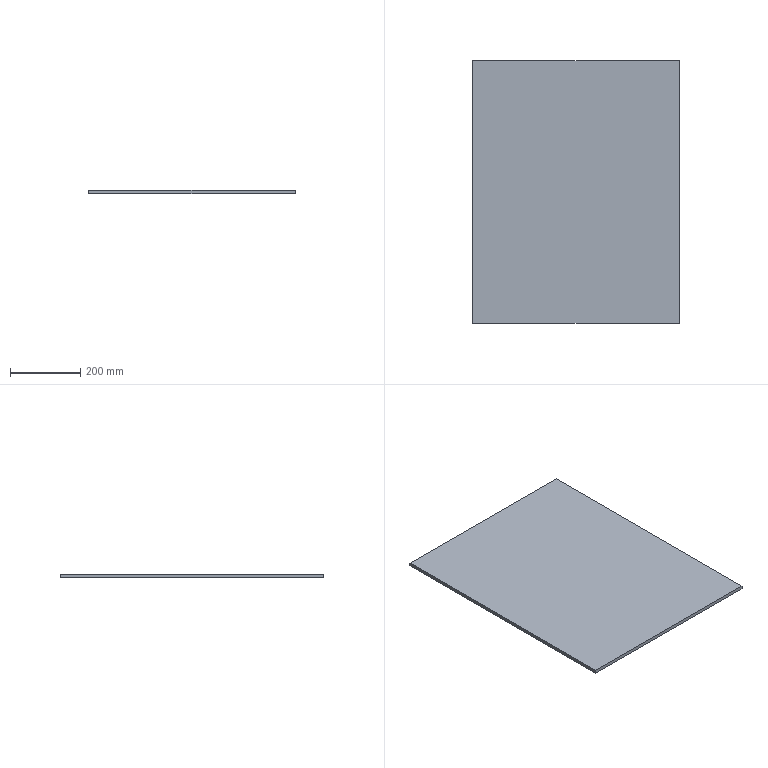Part | STEP file | floor | 1 solid | 6 faces | box 586.14 x 746.049 x 10 mm | volume 4372895 mm3 | plane 6
STEP:
#1=CARTESIAN_POINT('',(0.,0.,0.));
#2=DIRECTION('',(0.,0.,1.));
#3=DIRECTION('',(1.,0.,0.));
#4=AXIS2_PLACEMENT_3D('',#1,#2,#3);
#5=CARTESIAN_POINT('',(36.295,-184.35,-10.));
#6=VERTEX_POINT('',#5);
#7=CARTESIAN_POINT('',(36.295,561.699,-10.));
#8=VERTEX_POINT('',#7);
#9=CARTESIAN_POINT('',(36.295,-184.35,-10.));
#10=DIRECTION('',(0.,1.,0.));
#11=VECTOR('',#10,1.);
#12=LINE('',#9,#11);
#13=CARTESIAN_POINT('',(36.295,-184.35,0.));
#14=DIRECTION('',(1.,0.,0.));
#15=DIRECTION('',(0.,0.,-1.));
#16=AXIS2_PLACEMENT_3D('',#13,#14,#15);
#17=PLANE('',#16);
#18=CARTESIAN_POINT('',(10.,0.));
#19=DIRECTION('',(0.,1.));
#20=VECTOR('',#19,1.);
#21=LINE('',#18,#20);
#22=(GEOMETRIC_REPRESENTATION_CONTEXT(2)PARAMETRIC_REPRESENTATION_CONTEXT()REPRESENTATION_CONTEXT('',''));
#23=DEFINITIONAL_REPRESENTATION('',(#21),#22);
#24=PCURVE('',#17,#23);
#25=CARTESIAN_POINT('',(-256.775,188.674,-10.));
#26=DIRECTION('',(0.,0.,1.));
#27=DIRECTION('',(1.,0.,0.));
#28=AXIS2_PLACEMENT_3D('',#25,#26,#27);
#29=PLANE('',#28);
#30=CARTESIAN_POINT('',(293.07,-373.025));
#31=DIRECTION('',(0.,1.));
#32=VECTOR('',#31,1.);
#33=LINE('',#30,#32);
#34=(GEOMETRIC_REPRESENTATION_CONTEXT(2)PARAMETRIC_REPRESENTATION_CONTEXT()REPRESENTATION_CONTEXT('',''));
#35=DEFINITIONAL_REPRESENTATION('',(#33),#34);
#36=PCURVE('',#29,#35);
#37=SURFACE_CURVE('',#12,(#24,#36),.PCURVE_S1.);
#38=EDGE_CURVE('',#6,#8,#37,.T.);
#39=ORIENTED_EDGE('',*,*,#38,.T.);
#40=CARTESIAN_POINT('',(36.295,561.699,0.));
#41=VERTEX_POINT('',#40);
#42=CARTESIAN_POINT('',(36.295,561.699,0.));
#43=DIRECTION('',(0.,0.,-1.));
#44=VECTOR('',#43,1.);
#45=LINE('',#42,#44);
#46=CARTESIAN_POINT('',(0.,746.049));
#47=DIRECTION('',(1.,0.));
#48=VECTOR('',#47,1.);
#49=LINE('',#46,#48);
#50=(GEOMETRIC_REPRESENTATION_CONTEXT(2)PARAMETRIC_REPRESENTATION_CONTEXT()REPRESENTATION_CONTEXT('',''));
#51=DEFINITIONAL_REPRESENTATION('',(#49),#50);
#52=PCURVE('',#17,#51);
#53=CARTESIAN_POINT('',(36.295,561.699,0.));
#54=DIRECTION('',(0.,1.,0.));
#55=DIRECTION('',(0.,0.,1.));
#56=AXIS2_PLACEMENT_3D('',#53,#54,#55);
#57=PLANE('',#56);
#58=CARTESIAN_POINT('',(0.,0.));
#59=DIRECTION('',(-1.,0.));
#60=VECTOR('',#59,1.);
#61=LINE('',#58,#60);
#62=(GEOMETRIC_REPRESENTATION_CONTEXT(2)PARAMETRIC_REPRESENTATION_CONTEXT()REPRESENTATION_CONTEXT('',''));
#63=DEFINITIONAL_REPRESENTATION('',(#61),#62);
#64=PCURVE('',#57,#63);
#65=SURFACE_CURVE('',#45,(#52,#64),.PCURVE_S1.);
#66=EDGE_CURVE('',#41,#8,#65,.T.);
#67=ORIENTED_EDGE('',*,*,#66,.F.);
#68=CARTESIAN_POINT('',(36.295,-184.35,0.));
#69=VERTEX_POINT('',#68);
#70=CARTESIAN_POINT('',(36.295,561.699,0.));
#71=DIRECTION('',(0.,-1.,0.));
#72=VECTOR('',#71,1.);
#73=LINE('',#70,#72);
#74=CARTESIAN_POINT('',(0.,746.049));
#75=DIRECTION('',(0.,-1.));
#76=VECTOR('',#75,1.);
#77=LINE('',#74,#76);
#78=(GEOMETRIC_REPRESENTATION_CONTEXT(2)PARAMETRIC_REPRESENTATION_CONTEXT()REPRESENTATION_CONTEXT('',''));
#79=DEFINITIONAL_REPRESENTATION('',(#77),#78);
#80=PCURVE('',#17,#79);
#81=CARTESIAN_POINT('',(-256.775,188.674,0.));
#82=DIRECTION('',(0.,0.,1.));
#83=DIRECTION('',(1.,0.,0.));
#84=AXIS2_PLACEMENT_3D('',#81,#82,#83);
#85=PLANE('',#84);
#86=CARTESIAN_POINT('',(293.07,373.025));
#87=DIRECTION('',(0.,-1.));
#88=VECTOR('',#87,1.);
#89=LINE('',#86,#88);
#90=(GEOMETRIC_REPRESENTATION_CONTEXT(2)PARAMETRIC_REPRESENTATION_CONTEXT()REPRESENTATION_CONTEXT('',''));
#91=DEFINITIONAL_REPRESENTATION('',(#89),#90);
#92=PCURVE('',#85,#91);
#93=SURFACE_CURVE('',#73,(#80,#92),.PCURVE_S1.);
#94=EDGE_CURVE('',#41,#69,#93,.T.);
#95=ORIENTED_EDGE('',*,*,#94,.T.);
#96=CARTESIAN_POINT('',(36.295,-184.35,0.));
#97=DIRECTION('',(0.,0.,-1.));
#98=VECTOR('',#97,1.);
#99=LINE('',#96,#98);
#100=CARTESIAN_POINT('',(0.,0.));
#101=DIRECTION('',(1.,0.));
#102=VECTOR('',#101,1.);
#103=LINE('',#100,#102);
#104=(GEOMETRIC_REPRESENTATION_CONTEXT(2)PARAMETRIC_REPRESENTATION_CONTEXT()REPRESENTATION_CONTEXT('',''));
#105=DEFINITIONAL_REPRESENTATION('',(#103),#104);
#106=PCURVE('',#17,#105);
#107=CARTESIAN_POINT('',(-549.845,-184.35,0.));
#108=DIRECTION('',(0.,-1.,0.));
#109=DIRECTION('',(0.,0.,-1.));
#110=AXIS2_PLACEMENT_3D('',#107,#108,#109);
#111=PLANE('',#110);
#112=CARTESIAN_POINT('',(0.,586.14));
#113=DIRECTION('',(1.,0.));
#114=VECTOR('',#113,1.);
#115=LINE('',#112,#114);
#116=(GEOMETRIC_REPRESENTATION_CONTEXT(2)PARAMETRIC_REPRESENTATION_CONTEXT()REPRESENTATION_CONTEXT('',''));
#117=DEFINITIONAL_REPRESENTATION('',(#115),#116);
#118=PCURVE('',#111,#117);
#119=SURFACE_CURVE('',#99,(#106,#118),.PCURVE_S1.);
#120=EDGE_CURVE('',#69,#6,#119,.T.);
#121=ORIENTED_EDGE('',*,*,#120,.T.);
#122=EDGE_LOOP('',(#39,#67,#95,#121));
#123=FACE_BOUND('',#122,.T.);
#124=ADVANCED_FACE('',(#123),#17,.T.);
#125=CARTESIAN_POINT('',(-549.845,561.699,-10.));
#126=VERTEX_POINT('',#125);
#127=CARTESIAN_POINT('',(36.295,561.699,-10.));
#128=DIRECTION('',(-1.,0.,0.));
#129=VECTOR('',#128,1.);
#130=LINE('',#127,#129);
#131=CARTESIAN_POINT('',(-10.,0.));
#132=DIRECTION('',(0.,-1.));
#133=VECTOR('',#132,1.);
#134=LINE('',#131,#133);
#135=(GEOMETRIC_REPRESENTATION_CONTEXT(2)PARAMETRIC_REPRESENTATION_CONTEXT()REPRESENTATION_CONTEXT('',''));
#136=DEFINITIONAL_REPRESENTATION('',(#134),#135);
#137=PCURVE('',#57,#136);
#138=CARTESIAN_POINT('',(293.07,373.025));
#139=DIRECTION('',(-1.,0.));
#140=VECTOR('',#139,1.);
#141=LINE('',#138,#140);
#142=(GEOMETRIC_REPRESENTATION_CONTEXT(2)PARAMETRIC_REPRESENTATION_CONTEXT()REPRESENTATION_CONTEXT('',''));
#143=DEFINITIONAL_REPRESENTATION('',(#141),#142);
#144=PCURVE('',#29,#143);
#145=SURFACE_CURVE('',#130,(#137,#144),.PCURVE_S1.);
#146=EDGE_CURVE('',#8,#126,#145,.T.);
#147=ORIENTED_EDGE('',*,*,#146,.T.);
#148=CARTESIAN_POINT('',(-549.845,561.699,0.));
#149=VERTEX_POINT('',#148);
#150=CARTESIAN_POINT('',(-549.845,561.699,0.));
#151=DIRECTION('',(0.,0.,-1.));
#152=VECTOR('',#151,1.);
#153=LINE('',#150,#152);
#154=CARTESIAN_POINT('',(0.,-586.14));
#155=DIRECTION('',(-1.,0.));
#156=VECTOR('',#155,1.);
#157=LINE('',#154,#156);
#158=(GEOMETRIC_REPRESENTATION_CONTEXT(2)PARAMETRIC_REPRESENTATION_CONTEXT()REPRESENTATION_CONTEXT('',''));
#159=DEFINITIONAL_REPRESENTATION('',(#157),#158);
#160=PCURVE('',#57,#159);
#161=CARTESIAN_POINT('',(-549.845,561.699,0.));
#162=DIRECTION('',(-1.,0.,0.));
#163=DIRECTION('',(0.,0.,1.));
#164=AXIS2_PLACEMENT_3D('',#161,#162,#163);
#165=PLANE('',#164);
#166=CARTESIAN_POINT('',(0.,0.));
#167=DIRECTION('',(-1.,0.));
#168=VECTOR('',#167,1.);
#169=LINE('',#166,#168);
#170=(GEOMETRIC_REPRESENTATION_CONTEXT(2)PARAMETRIC_REPRESENTATION_CONTEXT()REPRESENTATION_CONTEXT('',''));
#171=DEFINITIONAL_REPRESENTATION('',(#169),#170);
#172=PCURVE('',#165,#171);
#173=SURFACE_CURVE('',#153,(#160,#172),.PCURVE_S1.);
#174=EDGE_CURVE('',#149,#126,#173,.T.);
#175=ORIENTED_EDGE('',*,*,#174,.F.);
#176=CARTESIAN_POINT('',(-549.845,561.699,0.));
#177=DIRECTION('',(1.,0.,0.));
#178=VECTOR('',#177,1.);
#179=LINE('',#176,#178);
#180=CARTESIAN_POINT('',(0.,-586.14));
#181=DIRECTION('',(0.,1.));
#182=VECTOR('',#181,1.);
#183=LINE('',#180,#182);
#184=(GEOMETRIC_REPRESENTATION_CONTEXT(2)PARAMETRIC_REPRESENTATION_CONTEXT()REPRESENTATION_CONTEXT('',''));
#185=DEFINITIONAL_REPRESENTATION('',(#183),#184);
#186=PCURVE('',#57,#185);
#187=CARTESIAN_POINT('',(-293.07,373.025));
#188=DIRECTION('',(1.,0.));
#189=VECTOR('',#188,1.);
#190=LINE('',#187,#189);
#191=(GEOMETRIC_REPRESENTATION_CONTEXT(2)PARAMETRIC_REPRESENTATION_CONTEXT()REPRESENTATION_CONTEXT('',''));
#192=DEFINITIONAL_REPRESENTATION('',(#190),#191);
#193=PCURVE('',#85,#192);
#194=SURFACE_CURVE('',#179,(#186,#193),.PCURVE_S1.);
#195=EDGE_CURVE('',#149,#41,#194,.T.);
#196=ORIENTED_EDGE('',*,*,#195,.T.);
#197=ORIENTED_EDGE('',*,*,#66,.T.);
#198=EDGE_LOOP('',(#147,#175,#196,#197));
#199=FACE_BOUND('',#198,.T.);
#200=ADVANCED_FACE('',(#199),#57,.T.);
#201=CARTESIAN_POINT('',(-549.845,-184.35,-10.));
#202=VERTEX_POINT('',#201);
#203=CARTESIAN_POINT('',(-549.845,561.699,-10.));
#204=DIRECTION('',(0.,-1.,0.));
#205=VECTOR('',#204,1.);
#206=LINE('',#203,#205);
#207=CARTESIAN_POINT('',(-10.,0.));
#208=DIRECTION('',(0.,-1.));
#209=VECTOR('',#208,1.);
#210=LINE('',#207,#209);
#211=(GEOMETRIC_REPRESENTATION_CONTEXT(2)PARAMETRIC_REPRESENTATION_CONTEXT()REPRESENTATION_CONTEXT('',''));
#212=DEFINITIONAL_REPRESENTATION('',(#210),#211);
#213=PCURVE('',#165,#212);
#214=CARTESIAN_POINT('',(-293.07,373.025));
#215=DIRECTION('',(0.,-1.));
#216=VECTOR('',#215,1.);
#217=LINE('',#214,#216);
#218=(GEOMETRIC_REPRESENTATION_CONTEXT(2)PARAMETRIC_REPRESENTATION_CONTEXT()REPRESENTATION_CONTEXT('',''));
#219=DEFINITIONAL_REPRESENTATION('',(#217),#218);
#220=PCURVE('',#29,#219);
#221=SURFACE_CURVE('',#206,(#213,#220),.PCURVE_S1.);
#222=EDGE_CURVE('',#126,#202,#221,.T.);
#223=ORIENTED_EDGE('',*,*,#222,.T.);
#224=CARTESIAN_POINT('',(-549.845,-184.35,0.));
#225=VERTEX_POINT('',#224);
#226=CARTESIAN_POINT('',(-549.845,-184.35,0.));
#227=DIRECTION('',(0.,0.,-1.));
#228=VECTOR('',#227,1.);
#229=LINE('',#226,#228);
#230=CARTESIAN_POINT('',(0.,-746.049));
#231=DIRECTION('',(-1.,0.));
#232=VECTOR('',#231,1.);
#233=LINE('',#230,#232);
#234=(GEOMETRIC_REPRESENTATION_CONTEXT(2)PARAMETRIC_REPRESENTATION_CONTEXT()REPRESENTATION_CONTEXT('',''));
#235=DEFINITIONAL_REPRESENTATION('',(#233),#234);
#236=PCURVE('',#165,#235);
#237=CARTESIAN_POINT('',(0.,0.));
#238=DIRECTION('',(1.,0.));
#239=VECTOR('',#238,1.);
#240=LINE('',#237,#239);
#241=(GEOMETRIC_REPRESENTATION_CONTEXT(2)PARAMETRIC_REPRESENTATION_CONTEXT()REPRESENTATION_CONTEXT('',''));
#242=DEFINITIONAL_REPRESENTATION('',(#240),#241);
#243=PCURVE('',#111,#242);
#244=SURFACE_CURVE('',#229,(#236,#243),.PCURVE_S1.);
#245=EDGE_CURVE('',#225,#202,#244,.T.);
#246=ORIENTED_EDGE('',*,*,#245,.F.);
#247=CARTESIAN_POINT('',(-549.845,-184.35,0.));
#248=DIRECTION('',(0.,1.,0.));
#249=VECTOR('',#248,1.);
#250=LINE('',#247,#249);
#251=CARTESIAN_POINT('',(0.,-746.049));
#252=DIRECTION('',(0.,1.));
#253=VECTOR('',#252,1.);
#254=LINE('',#251,#253);
#255=(GEOMETRIC_REPRESENTATION_CONTEXT(2)PARAMETRIC_REPRESENTATION_CONTEXT()REPRESENTATION_CONTEXT('',''));
#256=DEFINITIONAL_REPRESENTATION('',(#254),#255);
#257=PCURVE('',#165,#256);
#258=CARTESIAN_POINT('',(-293.07,-373.025));
#259=DIRECTION('',(0.,1.));
#260=VECTOR('',#259,1.);
#261=LINE('',#258,#260);
#262=(GEOMETRIC_REPRESENTATION_CONTEXT(2)PARAMETRIC_REPRESENTATION_CONTEXT()REPRESENTATION_CONTEXT('',''));
#263=DEFINITIONAL_REPRESENTATION('',(#261),#262);
#264=PCURVE('',#85,#263);
#265=SURFACE_CURVE('',#250,(#257,#264),.PCURVE_S1.);
#266=EDGE_CURVE('',#225,#149,#265,.T.);
#267=ORIENTED_EDGE('',*,*,#266,.T.);
#268=ORIENTED_EDGE('',*,*,#174,.T.);
#269=EDGE_LOOP('',(#223,#246,#267,#268));
#270=FACE_BOUND('',#269,.T.);
#271=ADVANCED_FACE('',(#270),#165,.T.);
#272=CARTESIAN_POINT('',(-549.845,-184.35,-10.));
#273=DIRECTION('',(1.,0.,0.));
#274=VECTOR('',#273,1.);
#275=LINE('',#272,#274);
#276=CARTESIAN_POINT('',(10.,0.));
#277=DIRECTION('',(0.,1.));
#278=VECTOR('',#277,1.);
#279=LINE('',#276,#278);
#280=(GEOMETRIC_REPRESENTATION_CONTEXT(2)PARAMETRIC_REPRESENTATION_CONTEXT()REPRESENTATION_CONTEXT('',''));
#281=DEFINITIONAL_REPRESENTATION('',(#279),#280);
#282=PCURVE('',#111,#281);
#283=CARTESIAN_POINT('',(-293.07,-373.025));
#284=DIRECTION('',(1.,0.));
#285=VECTOR('',#284,1.);
#286=LINE('',#283,#285);
#287=(GEOMETRIC_REPRESENTATION_CONTEXT(2)PARAMETRIC_REPRESENTATION_CONTEXT()REPRESENTATION_CONTEXT('',''));
#288=DEFINITIONAL_REPRESENTATION('',(#286),#287);
#289=PCURVE('',#29,#288);
#290=SURFACE_CURVE('',#275,(#282,#289),.PCURVE_S1.);
#291=EDGE_CURVE('',#202,#6,#290,.T.);
#292=ORIENTED_EDGE('',*,*,#291,.T.);
#293=ORIENTED_EDGE('',*,*,#120,.F.);
#294=CARTESIAN_POINT('',(36.295,-184.35,0.));
#295=DIRECTION('',(-1.,0.,0.));
#296=VECTOR('',#295,1.);
#297=LINE('',#294,#296);
#298=CARTESIAN_POINT('',(0.,586.14));
#299=DIRECTION('',(0.,-1.));
#300=VECTOR('',#299,1.);
#301=LINE('',#298,#300);
#302=(GEOMETRIC_REPRESENTATION_CONTEXT(2)PARAMETRIC_REPRESENTATION_CONTEXT()REPRESENTATION_CONTEXT('',''));
#303=DEFINITIONAL_REPRESENTATION('',(#301),#302);
#304=PCURVE('',#111,#303);
#305=CARTESIAN_POINT('',(293.07,-373.025));
#306=DIRECTION('',(-1.,0.));
#307=VECTOR('',#306,1.);
#308=LINE('',#305,#307);
#309=(GEOMETRIC_REPRESENTATION_CONTEXT(2)PARAMETRIC_REPRESENTATION_CONTEXT()REPRESENTATION_CONTEXT('',''));
#310=DEFINITIONAL_REPRESENTATION('',(#308),#309);
#311=PCURVE('',#85,#310);
#312=SURFACE_CURVE('',#297,(#304,#311),.PCURVE_S1.);
#313=EDGE_CURVE('',#69,#225,#312,.T.);
#314=ORIENTED_EDGE('',*,*,#313,.T.);
#315=ORIENTED_EDGE('',*,*,#245,.T.);
#316=EDGE_LOOP('',(#292,#293,#314,#315));
#317=FACE_BOUND('',#316,.T.);
#318=ADVANCED_FACE('',(#317),#111,.T.);
#319=ORIENTED_EDGE('',*,*,#313,.F.);
#320=ORIENTED_EDGE('',*,*,#94,.F.);
#321=ORIENTED_EDGE('',*,*,#195,.F.);
#322=ORIENTED_EDGE('',*,*,#266,.F.);
#323=EDGE_LOOP('',(#319,#320,#321,#322));
#324=FACE_BOUND('',#323,.T.);
#325=ADVANCED_FACE('',(#324),#85,.T.);
#326=ORIENTED_EDGE('',*,*,#38,.F.);
#327=ORIENTED_EDGE('',*,*,#291,.F.);
#328=ORIENTED_EDGE('',*,*,#222,.F.);
#329=ORIENTED_EDGE('',*,*,#146,.F.);
#330=EDGE_LOOP('',(#326,#327,#328,#329));
#331=FACE_BOUND('',#330,.T.);
#332=ADVANCED_FACE('',(#331),#29,.F.);
#333=CLOSED_SHELL('',(#124,#200,#271,#318,#325,#332));
#334=MANIFOLD_SOLID_BREP('',#333);
#335=(LENGTH_UNIT()NAMED_UNIT(*)SI_UNIT(.MILLI.,.METRE.));
#336=UNCERTAINTY_MEASURE_WITH_UNIT(LENGTH_MEASURE(0.0000001),#335,'','');
#337=(NAMED_UNIT(*)PLANE_ANGLE_UNIT()SI_UNIT($,.RADIAN.));
#338=(NAMED_UNIT(*)SI_UNIT($,.STERADIAN.)SOLID_ANGLE_UNIT());
#339=(GEOMETRIC_REPRESENTATION_CONTEXT(3)GLOBAL_UNCERTAINTY_ASSIGNED_CONTEXT((#336))GLOBAL_UNIT_ASSIGNED_CONTEXT((#335,#337,#338))REPRESENTATION_CONTEXT('',''));
#340=ADVANCED_BREP_SHAPE_REPRESENTATION('',(#4,#334),#339);